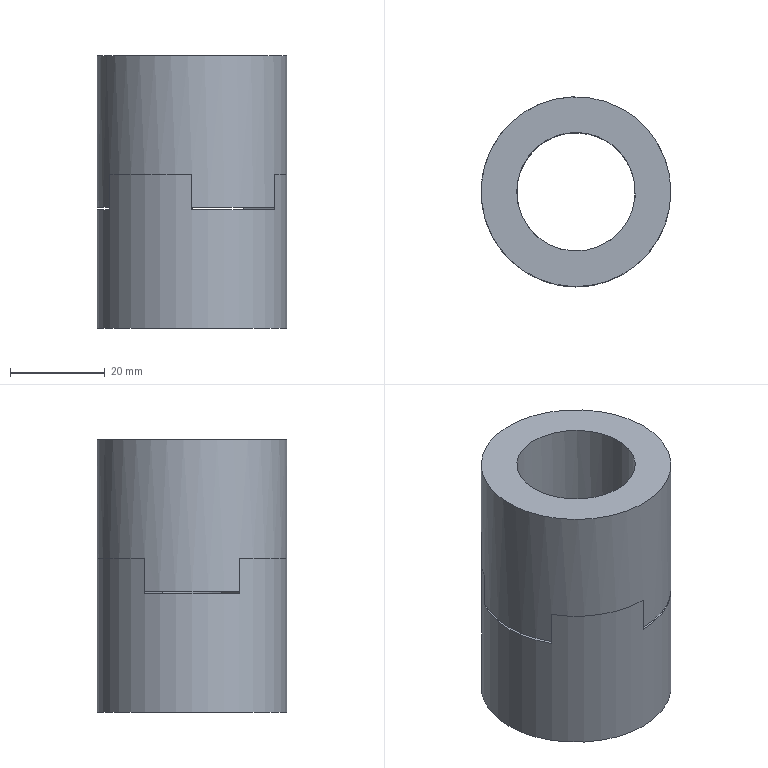Part | NX | 2 solids | 30 faces | box 40 x 40 x 57.5 mm | volume 43840 mm3 | plane 26 | cylinder 4 | commonest cylinder face diameters 25 x2 40 x2
STEP:
#1=CARTESIAN_POINT('',(740.769,-282.606,215.5));
#2=VERTEX_POINT('',#1);
#3=CARTESIAN_POINT('',(751.594,-276.356,215.5));
#4=VERTEX_POINT('',#3);
#5=CARTESIAN_POINT('',(751.594,-288.856,215.5));
#6=DIRECTION('',(0.,0.,-1.));
#7=DIRECTION('',(-1.,0.,0.));
#8=AXIS2_PLACEMENT_3D('',#5,#6,#7);
#9=CIRCLE('',#8,12.5);
#10=EDGE_CURVE('',#2,#4,#9,.T.);
#11=ORIENTED_EDGE('',*,*,#10,.F.);
#12=CARTESIAN_POINT('',(734.274,-278.856,215.5));
#13=VERTEX_POINT('',#12);
#14=CARTESIAN_POINT('',(734.274,-278.856,215.5));
#15=DIRECTION('',(0.866,-0.5,0.));
#16=VECTOR('',#15,1.);
#17=LINE('',#14,#16);
#18=EDGE_CURVE('',#13,#2,#17,.T.);
#19=ORIENTED_EDGE('',*,*,#18,.F.);
#20=CARTESIAN_POINT('',(751.594,-268.856,215.5));
#21=VERTEX_POINT('',#20);
#22=CARTESIAN_POINT('',(751.594,-288.856,215.5));
#23=DIRECTION('',(0.,0.,-1.));
#24=DIRECTION('',(-1.,0.,0.));
#25=AXIS2_PLACEMENT_3D('',#22,#23,#24);
#26=CIRCLE('',#25,20.);
#27=EDGE_CURVE('',#13,#21,#26,.T.);
#28=ORIENTED_EDGE('',*,*,#27,.T.);
#29=CARTESIAN_POINT('',(751.594,-276.356,215.5));
#30=DIRECTION('',(0.,1.,0.));
#31=VECTOR('',#30,1.);
#32=LINE('',#29,#31);
#33=EDGE_CURVE('',#4,#21,#32,.T.);
#34=ORIENTED_EDGE('',*,*,#33,.F.);
#35=EDGE_LOOP('',(#11,#19,#28,#34));
#36=FACE_OUTER_BOUND('',#35,.T.);
#37=CARTESIAN_POINT('',(751.594,-288.856,215.5));
#38=DIRECTION('',(0.,0.,-1.));
#39=DIRECTION('',(1.,0.,0.));
#40=AXIS2_PLACEMENT_3D('',#37,#38,#39);
#41=PLANE('',#40);
#42=ADVANCED_FACE('',(#36),#41,.T.);
#43=CARTESIAN_POINT('',(762.42,-282.606,215.5));
#44=VERTEX_POINT('',#43);
#45=CARTESIAN_POINT('',(762.42,-295.106,215.5));
#46=VERTEX_POINT('',#45);
#47=CARTESIAN_POINT('',(751.594,-288.856,215.5));
#48=DIRECTION('',(0.,0.,-1.));
#49=DIRECTION('',(-1.,0.,0.));
#50=AXIS2_PLACEMENT_3D('',#47,#48,#49);
#51=CIRCLE('',#50,12.5);
#52=EDGE_CURVE('',#44,#46,#51,.T.);
#53=ORIENTED_EDGE('',*,*,#52,.F.);
#54=CARTESIAN_POINT('',(768.915,-278.856,215.5));
#55=VERTEX_POINT('',#54);
#56=CARTESIAN_POINT('',(768.915,-278.856,215.5));
#57=DIRECTION('',(-0.866,-0.5,0.));
#58=VECTOR('',#57,1.);
#59=LINE('',#56,#58);
#60=EDGE_CURVE('',#55,#44,#59,.T.);
#61=ORIENTED_EDGE('',*,*,#60,.F.);
#62=CARTESIAN_POINT('',(768.915,-298.856,215.5));
#63=VERTEX_POINT('',#62);
#64=CARTESIAN_POINT('',(751.594,-288.856,215.5));
#65=DIRECTION('',(0.,0.,-1.));
#66=DIRECTION('',(-1.,0.,0.));
#67=AXIS2_PLACEMENT_3D('',#64,#65,#66);
#68=CIRCLE('',#67,20.);
#69=EDGE_CURVE('',#55,#63,#68,.T.);
#70=ORIENTED_EDGE('',*,*,#69,.T.);
#71=CARTESIAN_POINT('',(762.42,-295.106,215.5));
#72=DIRECTION('',(0.866,-0.5,0.));
#73=VECTOR('',#72,1.);
#74=LINE('',#71,#73);
#75=EDGE_CURVE('',#46,#63,#74,.T.);
#76=ORIENTED_EDGE('',*,*,#75,.F.);
#77=EDGE_LOOP('',(#53,#61,#70,#76));
#78=FACE_OUTER_BOUND('',#77,.T.);
#79=CARTESIAN_POINT('',(751.594,-288.856,215.5));
#80=DIRECTION('',(0.,0.,-1.));
#81=DIRECTION('',(1.,0.,0.));
#82=AXIS2_PLACEMENT_3D('',#79,#80,#81);
#83=PLANE('',#82);
#84=ADVANCED_FACE('',(#78),#83,.T.);
#85=CARTESIAN_POINT('',(751.594,-301.356,215.5));
#86=VERTEX_POINT('',#85);
#87=CARTESIAN_POINT('',(740.769,-295.106,215.5));
#88=VERTEX_POINT('',#87);
#89=CARTESIAN_POINT('',(751.594,-288.856,215.5));
#90=DIRECTION('',(0.,0.,-1.));
#91=DIRECTION('',(-1.,0.,0.));
#92=AXIS2_PLACEMENT_3D('',#89,#90,#91);
#93=CIRCLE('',#92,12.5);
#94=EDGE_CURVE('',#86,#88,#93,.T.);
#95=ORIENTED_EDGE('',*,*,#94,.F.);
#96=CARTESIAN_POINT('',(751.594,-308.856,215.5));
#97=VERTEX_POINT('',#96);
#98=CARTESIAN_POINT('',(751.594,-308.856,215.5));
#99=DIRECTION('',(0.,1.,0.));
#100=VECTOR('',#99,1.);
#101=LINE('',#98,#100);
#102=EDGE_CURVE('',#97,#86,#101,.T.);
#103=ORIENTED_EDGE('',*,*,#102,.F.);
#104=CARTESIAN_POINT('',(734.274,-298.856,215.5));
#105=VERTEX_POINT('',#104);
#106=CARTESIAN_POINT('',(751.594,-288.856,215.5));
#107=DIRECTION('',(0.,0.,-1.));
#108=DIRECTION('',(-1.,0.,0.));
#109=AXIS2_PLACEMENT_3D('',#106,#107,#108);
#110=CIRCLE('',#109,20.);
#111=EDGE_CURVE('',#97,#105,#110,.T.);
#112=ORIENTED_EDGE('',*,*,#111,.T.);
#113=CARTESIAN_POINT('',(740.769,-295.106,215.5));
#114=DIRECTION('',(-0.866,-0.5,0.));
#115=VECTOR('',#114,1.);
#116=LINE('',#113,#115);
#117=EDGE_CURVE('',#88,#105,#116,.T.);
#118=ORIENTED_EDGE('',*,*,#117,.F.);
#119=EDGE_LOOP('',(#95,#103,#112,#118));
#120=FACE_OUTER_BOUND('',#119,.T.);
#121=CARTESIAN_POINT('',(751.594,-288.856,215.5));
#122=DIRECTION('',(0.,0.,-1.));
#123=DIRECTION('',(1.,0.,0.));
#124=AXIS2_PLACEMENT_3D('',#121,#122,#123);
#125=PLANE('',#124);
#126=ADVANCED_FACE('',(#120),#125,.T.);
#127=CARTESIAN_POINT('',(771.594,-288.856,240.5));
#128=VERTEX_POINT('',#127);
#129=CARTESIAN_POINT('',(751.594,-288.856,240.5));
#130=DIRECTION('',(0.,0.,1.));
#131=DIRECTION('',(1.,0.,0.));
#132=AXIS2_PLACEMENT_3D('',#129,#130,#131);
#133=CIRCLE('',#132,20.);
#134=EDGE_CURVE('',#128,#128,#133,.T.);
#135=ORIENTED_EDGE('',*,*,#134,.F.);
#136=EDGE_LOOP('',(#135));
#137=FACE_BOUND('',#136,.T.);
#138=ORIENTED_EDGE('',*,*,#111,.F.);
#139=CARTESIAN_POINT('',(751.594,-308.856,208.5));
#140=VERTEX_POINT('',#139);
#141=CARTESIAN_POINT('',(751.594,-308.856,215.5));
#142=DIRECTION('',(0.,0.,-1.));
#143=VECTOR('',#142,1.);
#144=LINE('',#141,#143);
#145=EDGE_CURVE('',#97,#140,#144,.T.);
#146=ORIENTED_EDGE('',*,*,#145,.T.);
#147=CARTESIAN_POINT('',(768.915,-298.856,208.5));
#148=VERTEX_POINT('',#147);
#149=CARTESIAN_POINT('',(751.594,-288.856,208.5));
#150=DIRECTION('',(0.,0.,1.));
#151=DIRECTION('',(1.,0.,0.));
#152=AXIS2_PLACEMENT_3D('',#149,#150,#151);
#153=CIRCLE('',#152,20.);
#154=EDGE_CURVE('',#140,#148,#153,.T.);
#155=ORIENTED_EDGE('',*,*,#154,.T.);
#156=CARTESIAN_POINT('',(768.915,-298.856,215.5));
#157=DIRECTION('',(0.,0.,-1.));
#158=VECTOR('',#157,1.);
#159=LINE('',#156,#158);
#160=EDGE_CURVE('',#63,#148,#159,.T.);
#161=ORIENTED_EDGE('',*,*,#160,.F.);
#162=ORIENTED_EDGE('',*,*,#69,.F.);
#163=CARTESIAN_POINT('',(768.915,-278.856,208.5));
#164=VERTEX_POINT('',#163);
#165=CARTESIAN_POINT('',(768.915,-278.856,215.5));
#166=DIRECTION('',(0.,0.,-1.));
#167=VECTOR('',#166,1.);
#168=LINE('',#165,#167);
#169=EDGE_CURVE('',#55,#164,#168,.T.);
#170=ORIENTED_EDGE('',*,*,#169,.T.);
#171=CARTESIAN_POINT('',(751.594,-268.856,208.5));
#172=VERTEX_POINT('',#171);
#173=CARTESIAN_POINT('',(751.594,-288.856,208.5));
#174=DIRECTION('',(0.,0.,1.));
#175=DIRECTION('',(1.,0.,0.));
#176=AXIS2_PLACEMENT_3D('',#173,#174,#175);
#177=CIRCLE('',#176,20.);
#178=EDGE_CURVE('',#164,#172,#177,.T.);
#179=ORIENTED_EDGE('',*,*,#178,.T.);
#180=CARTESIAN_POINT('',(751.594,-268.856,215.5));
#181=DIRECTION('',(0.,0.,-1.));
#182=VECTOR('',#181,1.);
#183=LINE('',#180,#182);
#184=EDGE_CURVE('',#21,#172,#183,.T.);
#185=ORIENTED_EDGE('',*,*,#184,.F.);
#186=ORIENTED_EDGE('',*,*,#27,.F.);
#187=CARTESIAN_POINT('',(734.274,-278.856,208.5));
#188=VERTEX_POINT('',#187);
#189=CARTESIAN_POINT('',(734.274,-278.856,215.5));
#190=DIRECTION('',(0.,0.,-1.));
#191=VECTOR('',#190,1.);
#192=LINE('',#189,#191);
#193=EDGE_CURVE('',#13,#188,#192,.T.);
#194=ORIENTED_EDGE('',*,*,#193,.T.);
#195=CARTESIAN_POINT('',(734.274,-298.856,208.5));
#196=VERTEX_POINT('',#195);
#197=CARTESIAN_POINT('',(751.594,-288.856,208.5));
#198=DIRECTION('',(0.,0.,1.));
#199=DIRECTION('',(1.,0.,0.));
#200=AXIS2_PLACEMENT_3D('',#197,#198,#199);
#201=CIRCLE('',#200,20.);
#202=EDGE_CURVE('',#188,#196,#201,.T.);
#203=ORIENTED_EDGE('',*,*,#202,.T.);
#204=CARTESIAN_POINT('',(734.274,-298.856,215.5));
#205=DIRECTION('',(0.,0.,-1.));
#206=VECTOR('',#205,1.);
#207=LINE('',#204,#206);
#208=EDGE_CURVE('',#105,#196,#207,.T.);
#209=ORIENTED_EDGE('',*,*,#208,.F.);
#210=EDGE_LOOP('',(#138,#146,#155,#161,#162,#170,#179,#185,#186,#194,#203,#209));
#211=FACE_BOUND('',#210,.T.);
#212=CARTESIAN_POINT('',(751.594,-288.856,240.5));
#213=DIRECTION('',(0.,0.,-1.));
#214=DIRECTION('',(1.,0.,0.));
#215=AXIS2_PLACEMENT_3D('',#212,#213,#214);
#216=CYLINDRICAL_SURFACE('',#215,20.);
#217=ADVANCED_FACE('',(#137,#211),#216,.T.);
#218=CARTESIAN_POINT('',(739.094,-288.856,240.5));
#219=VERTEX_POINT('',#218);
#220=CARTESIAN_POINT('',(751.594,-288.856,240.5));
#221=DIRECTION('',(0.,0.,-1.));
#222=DIRECTION('',(-1.,0.,0.));
#223=AXIS2_PLACEMENT_3D('',#220,#221,#222);
#224=CIRCLE('',#223,12.5);
#225=EDGE_CURVE('',#219,#219,#224,.T.);
#226=ORIENTED_EDGE('',*,*,#225,.T.);
#227=EDGE_LOOP('',(#226));
#228=FACE_BOUND('',#227,.T.);
#229=ORIENTED_EDGE('',*,*,#134,.T.);
#230=EDGE_LOOP('',(#229));
#231=FACE_BOUND('',#230,.T.);
#232=CARTESIAN_POINT('',(751.594,-288.856,240.5));
#233=DIRECTION('',(0.,0.,1.));
#234=DIRECTION('',(-1.,0.,0.));
#235=AXIS2_PLACEMENT_3D('',#232,#233,#234);
#236=PLANE('',#235);
#237=ADVANCED_FACE('',(#228,#231),#236,.T.);
#238=CARTESIAN_POINT('',(751.594,-301.356,208.5));
#239=VERTEX_POINT('',#238);
#240=CARTESIAN_POINT('',(751.594,-308.856,208.5));
#241=DIRECTION('',(0.,1.,0.));
#242=VECTOR('',#241,1.);
#243=LINE('',#240,#242);
#244=EDGE_CURVE('',#140,#239,#243,.T.);
#245=ORIENTED_EDGE('',*,*,#244,.F.);
#246=ORIENTED_EDGE('',*,*,#145,.F.);
#247=ORIENTED_EDGE('',*,*,#102,.T.);
#248=CARTESIAN_POINT('',(751.594,-301.356,215.5));
#249=DIRECTION('',(0.,0.,-1.));
#250=VECTOR('',#249,1.);
#251=LINE('',#248,#250);
#252=EDGE_CURVE('',#86,#239,#251,.T.);
#253=ORIENTED_EDGE('',*,*,#252,.T.);
#254=EDGE_LOOP('',(#245,#246,#247,#253));
#255=FACE_OUTER_BOUND('',#254,.T.);
#256=CARTESIAN_POINT('',(751.594,-308.856,215.5));
#257=DIRECTION('',(-1.,0.,0.));
#258=DIRECTION('',(0.,0.,-1.));
#259=AXIS2_PLACEMENT_3D('',#256,#257,#258);
#260=PLANE('',#259);
#261=ADVANCED_FACE('',(#255),#260,.T.);
#262=CARTESIAN_POINT('',(762.42,-295.106,208.5));
#263=VERTEX_POINT('',#262);
#264=CARTESIAN_POINT('',(762.42,-295.106,208.5));
#265=DIRECTION('',(0.866,-0.5,0.));
#266=VECTOR('',#265,1.);
#267=LINE('',#264,#266);
#268=EDGE_CURVE('',#263,#148,#267,.T.);
#269=ORIENTED_EDGE('',*,*,#268,.F.);
#270=CARTESIAN_POINT('',(762.42,-295.106,215.5));
#271=DIRECTION('',(0.,0.,-1.));
#272=VECTOR('',#271,1.);
#273=LINE('',#270,#272);
#274=EDGE_CURVE('',#46,#263,#273,.T.);
#275=ORIENTED_EDGE('',*,*,#274,.F.);
#276=ORIENTED_EDGE('',*,*,#75,.T.);
#277=ORIENTED_EDGE('',*,*,#160,.T.);
#278=EDGE_LOOP('',(#269,#275,#276,#277));
#279=FACE_OUTER_BOUND('',#278,.T.);
#280=CARTESIAN_POINT('',(762.42,-295.106,215.5));
#281=DIRECTION('',(0.5,0.866,0.));
#282=DIRECTION('',(0.866,-0.5,0.));
#283=AXIS2_PLACEMENT_3D('',#280,#281,#282);
#284=PLANE('',#283);
#285=ADVANCED_FACE('',(#279),#284,.T.);
#286=CARTESIAN_POINT('',(751.594,-288.856,208.5));
#287=DIRECTION('',(0.,0.,1.));
#288=DIRECTION('',(1.,0.,0.));
#289=AXIS2_PLACEMENT_3D('',#286,#287,#288);
#290=CIRCLE('',#289,12.5);
#291=EDGE_CURVE('',#239,#263,#290,.T.);
#292=ORIENTED_EDGE('',*,*,#291,.F.);
#293=ORIENTED_EDGE('',*,*,#252,.F.);
#294=ORIENTED_EDGE('',*,*,#94,.T.);
#295=CARTESIAN_POINT('',(740.769,-295.106,208.5));
#296=VERTEX_POINT('',#295);
#297=CARTESIAN_POINT('',(740.769,-295.106,215.5));
#298=DIRECTION('',(0.,0.,-1.));
#299=VECTOR('',#298,1.);
#300=LINE('',#297,#299);
#301=EDGE_CURVE('',#88,#296,#300,.T.);
#302=ORIENTED_EDGE('',*,*,#301,.T.);
#303=CARTESIAN_POINT('',(740.769,-282.606,208.5));
#304=VERTEX_POINT('',#303);
#305=CARTESIAN_POINT('',(751.594,-288.856,208.5));
#306=DIRECTION('',(0.,0.,1.));
#307=DIRECTION('',(1.,0.,0.));
#308=AXIS2_PLACEMENT_3D('',#305,#306,#307);
#309=CIRCLE('',#308,12.5);
#310=EDGE_CURVE('',#304,#296,#309,.T.);
#311=ORIENTED_EDGE('',*,*,#310,.F.);
#312=CARTESIAN_POINT('',(740.769,-282.606,215.5));
#313=DIRECTION('',(0.,0.,-1.));
#314=VECTOR('',#313,1.);
#315=LINE('',#312,#314);
#316=EDGE_CURVE('',#2,#304,#315,.T.);
#317=ORIENTED_EDGE('',*,*,#316,.F.);
#318=ORIENTED_EDGE('',*,*,#10,.T.);
#319=CARTESIAN_POINT('',(751.594,-276.356,208.5));
#320=VERTEX_POINT('',#319);
#321=CARTESIAN_POINT('',(751.594,-276.356,215.5));
#322=DIRECTION('',(0.,0.,-1.));
#323=VECTOR('',#322,1.);
#324=LINE('',#321,#323);
#325=EDGE_CURVE('',#4,#320,#324,.T.);
#326=ORIENTED_EDGE('',*,*,#325,.T.);
#327=CARTESIAN_POINT('',(762.42,-282.606,208.5));
#328=VERTEX_POINT('',#327);
#329=CARTESIAN_POINT('',(751.594,-288.856,208.5));
#330=DIRECTION('',(0.,0.,1.));
#331=DIRECTION('',(1.,0.,0.));
#332=AXIS2_PLACEMENT_3D('',#329,#330,#331);
#333=CIRCLE('',#332,12.5);
#334=EDGE_CURVE('',#328,#320,#333,.T.);
#335=ORIENTED_EDGE('',*,*,#334,.F.);
#336=CARTESIAN_POINT('',(762.42,-282.606,215.5));
#337=DIRECTION('',(0.,0.,-1.));
#338=VECTOR('',#337,1.);
#339=LINE('',#336,#338);
#340=EDGE_CURVE('',#44,#328,#339,.T.);
#341=ORIENTED_EDGE('',*,*,#340,.F.);
#342=ORIENTED_EDGE('',*,*,#52,.T.);
#343=ORIENTED_EDGE('',*,*,#274,.T.);
#344=EDGE_LOOP('',(#292,#293,#294,#302,#311,#317,#318,#326,#335,#341,#342,#343));
#345=FACE_BOUND('',#344,.T.);
#346=ORIENTED_EDGE('',*,*,#225,.F.);
#347=EDGE_LOOP('',(#346));
#348=FACE_BOUND('',#347,.T.);
#349=CARTESIAN_POINT('',(751.594,-288.856,215.5));
#350=DIRECTION('',(0.,0.,-1.));
#351=DIRECTION('',(1.,0.,0.));
#352=AXIS2_PLACEMENT_3D('',#349,#350,#351);
#353=CYLINDRICAL_SURFACE('',#352,12.5);
#354=ADVANCED_FACE('',(#345,#348),#353,.F.);
#355=ORIENTED_EDGE('',*,*,#244,.T.);
#356=ORIENTED_EDGE('',*,*,#291,.T.);
#357=ORIENTED_EDGE('',*,*,#268,.T.);
#358=ORIENTED_EDGE('',*,*,#154,.F.);
#359=EDGE_LOOP('',(#355,#356,#357,#358));
#360=FACE_OUTER_BOUND('',#359,.T.);
#361=CARTESIAN_POINT('',(751.594,-288.856,208.5));
#362=DIRECTION('',(0.,0.,1.));
#363=DIRECTION('',(-1.,0.,0.));
#364=AXIS2_PLACEMENT_3D('',#361,#362,#363);
#365=PLANE('',#364);
#366=ADVANCED_FACE('',(#360),#365,.F.);
#367=CARTESIAN_POINT('',(740.769,-295.106,208.5));
#368=DIRECTION('',(-0.866,-0.5,0.));
#369=VECTOR('',#368,1.);
#370=LINE('',#367,#369);
#371=EDGE_CURVE('',#296,#196,#370,.T.);
#372=ORIENTED_EDGE('',*,*,#371,.F.);
#373=ORIENTED_EDGE('',*,*,#301,.F.);
#374=ORIENTED_EDGE('',*,*,#117,.T.);
#375=ORIENTED_EDGE('',*,*,#208,.T.);
#376=EDGE_LOOP('',(#372,#373,#374,#375));
#377=FACE_OUTER_BOUND('',#376,.T.);
#378=CARTESIAN_POINT('',(740.769,-295.106,215.5));
#379=DIRECTION('',(0.5,-0.866,0.));
#380=DIRECTION('',(-0.866,-0.5,0.));
#381=AXIS2_PLACEMENT_3D('',#378,#379,#380);
#382=PLANE('',#381);
#383=ADVANCED_FACE('',(#377),#382,.T.);
#384=CARTESIAN_POINT('',(734.274,-278.856,208.5));
#385=DIRECTION('',(0.866,-0.5,0.));
#386=VECTOR('',#385,1.);
#387=LINE('',#384,#386);
#388=EDGE_CURVE('',#188,#304,#387,.T.);
#389=ORIENTED_EDGE('',*,*,#388,.F.);
#390=ORIENTED_EDGE('',*,*,#193,.F.);
#391=ORIENTED_EDGE('',*,*,#18,.T.);
#392=ORIENTED_EDGE('',*,*,#316,.T.);
#393=EDGE_LOOP('',(#389,#390,#391,#392));
#394=FACE_OUTER_BOUND('',#393,.T.);
#395=CARTESIAN_POINT('',(734.274,-278.856,215.5));
#396=DIRECTION('',(0.5,0.866,0.));
#397=DIRECTION('',(0.866,-0.5,0.));
#398=AXIS2_PLACEMENT_3D('',#395,#396,#397);
#399=PLANE('',#398);
#400=ADVANCED_FACE('',(#394),#399,.T.);
#401=ORIENTED_EDGE('',*,*,#371,.T.);
#402=ORIENTED_EDGE('',*,*,#202,.F.);
#403=ORIENTED_EDGE('',*,*,#388,.T.);
#404=ORIENTED_EDGE('',*,*,#310,.T.);
#405=EDGE_LOOP('',(#401,#402,#403,#404));
#406=FACE_OUTER_BOUND('',#405,.T.);
#407=CARTESIAN_POINT('',(751.594,-288.856,208.5));
#408=DIRECTION('',(0.,0.,1.));
#409=DIRECTION('',(-1.,0.,0.));
#410=AXIS2_PLACEMENT_3D('',#407,#408,#409);
#411=PLANE('',#410);
#412=ADVANCED_FACE('',(#406),#411,.F.);
#413=CARTESIAN_POINT('',(751.594,-276.356,208.5));
#414=DIRECTION('',(0.,1.,0.));
#415=VECTOR('',#414,1.);
#416=LINE('',#413,#415);
#417=EDGE_CURVE('',#320,#172,#416,.T.);
#418=ORIENTED_EDGE('',*,*,#417,.F.);
#419=ORIENTED_EDGE('',*,*,#325,.F.);
#420=ORIENTED_EDGE('',*,*,#33,.T.);
#421=ORIENTED_EDGE('',*,*,#184,.T.);
#422=EDGE_LOOP('',(#418,#419,#420,#421));
#423=FACE_OUTER_BOUND('',#422,.T.);
#424=CARTESIAN_POINT('',(751.594,-276.356,215.5));
#425=DIRECTION('',(-1.,0.,0.));
#426=DIRECTION('',(0.,0.,-1.));
#427=AXIS2_PLACEMENT_3D('',#424,#425,#426);
#428=PLANE('',#427);
#429=ADVANCED_FACE('',(#423),#428,.T.);
#430=CARTESIAN_POINT('',(768.915,-278.856,208.5));
#431=DIRECTION('',(-0.866,-0.5,0.));
#432=VECTOR('',#431,1.);
#433=LINE('',#430,#432);
#434=EDGE_CURVE('',#164,#328,#433,.T.);
#435=ORIENTED_EDGE('',*,*,#434,.F.);
#436=ORIENTED_EDGE('',*,*,#169,.F.);
#437=ORIENTED_EDGE('',*,*,#60,.T.);
#438=ORIENTED_EDGE('',*,*,#340,.T.);
#439=EDGE_LOOP('',(#435,#436,#437,#438));
#440=FACE_OUTER_BOUND('',#439,.T.);
#441=CARTESIAN_POINT('',(768.915,-278.856,215.5));
#442=DIRECTION('',(0.5,-0.866,0.));
#443=DIRECTION('',(-0.866,-0.5,0.));
#444=AXIS2_PLACEMENT_3D('',#441,#442,#443);
#445=PLANE('',#444);
#446=ADVANCED_FACE('',(#440),#445,.T.);
#447=ORIENTED_EDGE('',*,*,#417,.T.);
#448=ORIENTED_EDGE('',*,*,#178,.F.);
#449=ORIENTED_EDGE('',*,*,#434,.T.);
#450=ORIENTED_EDGE('',*,*,#334,.T.);
#451=EDGE_LOOP('',(#447,#448,#449,#450));
#452=FACE_OUTER_BOUND('',#451,.T.);
#453=CARTESIAN_POINT('',(751.594,-288.856,208.5));
#454=DIRECTION('',(0.,0.,1.));
#455=DIRECTION('',(-1.,0.,0.));
#456=AXIS2_PLACEMENT_3D('',#453,#454,#455);
#457=PLANE('',#456);
#458=ADVANCED_FACE('',(#452),#457,.F.);
#459=CLOSED_SHELL('',(#42,#84,#126,#217,#237,#261,#285,#354,#366,#383,#400,#412,#429,#446,#458));
#460=MANIFOLD_SOLID_BREP('',#459);
#461=CARTESIAN_POINT('',(740.769,-295.106,208.));
#462=VERTEX_POINT('',#461);
#463=CARTESIAN_POINT('',(734.274,-298.856,208.));
#464=VERTEX_POINT('',#463);
#465=CARTESIAN_POINT('',(740.769,-295.106,208.));
#466=DIRECTION('',(-0.866,-0.5,0.));
#467=VECTOR('',#466,1.);
#468=LINE('',#465,#467);
#469=EDGE_CURVE('',#462,#464,#468,.T.);
#470=ORIENTED_EDGE('',*,*,#469,.F.);
#471=CARTESIAN_POINT('',(740.769,-282.606,208.));
#472=VERTEX_POINT('',#471);
#473=CARTESIAN_POINT('',(751.594,-288.856,208.));
#474=DIRECTION('',(0.,0.,1.));
#475=DIRECTION('',(1.,0.,0.));
#476=AXIS2_PLACEMENT_3D('',#473,#474,#475);
#477=CIRCLE('',#476,12.5);
#478=EDGE_CURVE('',#472,#462,#477,.T.);
#479=ORIENTED_EDGE('',*,*,#478,.F.);
#480=CARTESIAN_POINT('',(734.274,-278.856,208.));
#481=VERTEX_POINT('',#480);
#482=CARTESIAN_POINT('',(734.274,-278.856,208.));
#483=DIRECTION('',(0.866,-0.5,0.));
#484=VECTOR('',#483,1.);
#485=LINE('',#482,#484);
#486=EDGE_CURVE('',#481,#472,#485,.T.);
#487=ORIENTED_EDGE('',*,*,#486,.F.);
#488=CARTESIAN_POINT('',(751.594,-288.856,208.));
#489=DIRECTION('',(0.,0.,1.));
#490=DIRECTION('',(1.,0.,0.));
#491=AXIS2_PLACEMENT_3D('',#488,#489,#490);
#492=CIRCLE('',#491,20.);
#493=EDGE_CURVE('',#481,#464,#492,.T.);
#494=ORIENTED_EDGE('',*,*,#493,.T.);
#495=EDGE_LOOP('',(#470,#479,#487,#494));
#496=FACE_OUTER_BOUND('',#495,.T.);
#497=CARTESIAN_POINT('',(751.594,-288.856,208.));
#498=DIRECTION('',(0.,0.,1.));
#499=DIRECTION('',(-1.,0.,0.));
#500=AXIS2_PLACEMENT_3D('',#497,#498,#499);
#501=PLANE('',#500);
#502=ADVANCED_FACE('',(#496),#501,.T.);
#503=CARTESIAN_POINT('',(751.594,-308.856,208.));
#504=VERTEX_POINT('',#503);
#505=CARTESIAN_POINT('',(751.594,-301.356,208.));
#506=VERTEX_POINT('',#505);
#507=CARTESIAN_POINT('',(751.594,-308.856,208.));
#508=DIRECTION('',(0.,1.,0.));
#509=VECTOR('',#508,1.);
#510=LINE('',#507,#509);
#511=EDGE_CURVE('',#504,#506,#510,.T.);
#512=ORIENTED_EDGE('',*,*,#511,.F.);
#513=CARTESIAN_POINT('',(768.915,-298.856,208.));
#514=VERTEX_POINT('',#513);
#515=CARTESIAN_POINT('',(751.594,-288.856,208.));
#516=DIRECTION('',(0.,0.,1.));
#517=DIRECTION('',(1.,0.,0.));
#518=AXIS2_PLACEMENT_3D('',#515,#516,#517);
#519=CIRCLE('',#518,20.);
#520=EDGE_CURVE('',#504,#514,#519,.T.);
#521=ORIENTED_EDGE('',*,*,#520,.T.);
#522=CARTESIAN_POINT('',(762.42,-295.106,208.));
#523=VERTEX_POINT('',#522);
#524=CARTESIAN_POINT('',(762.42,-295.106,208.));
#525=DIRECTION('',(0.866,-0.5,0.));
#526=VECTOR('',#525,1.);
#527=LINE('',#524,#526);
#528=EDGE_CURVE('',#523,#514,#527,.T.);
#529=ORIENTED_EDGE('',*,*,#528,.F.);
#530=CARTESIAN_POINT('',(751.594,-288.856,208.));
#531=DIRECTION('',(0.,0.,1.));
#532=DIRECTION('',(1.,0.,0.));
#533=AXIS2_PLACEMENT_3D('',#530,#531,#532);
#534=CIRCLE('',#533,12.5);
#535=EDGE_CURVE('',#506,#523,#534,.T.);
#536=ORIENTED_EDGE('',*,*,#535,.F.);
#537=EDGE_LOOP('',(#512,#521,#529,#536));
#538=FACE_OUTER_BOUND('',#537,.T.);
#539=CARTESIAN_POINT('',(751.594,-288.856,208.));
#540=DIRECTION('',(0.,0.,1.));
#541=DIRECTION('',(-1.,0.,0.));
#542=AXIS2_PLACEMENT_3D('',#539,#540,#541);
#543=PLANE('',#542);
#544=ADVANCED_FACE('',(#538),#543,.T.);
#545=CARTESIAN_POINT('',(751.594,-276.356,208.));
#546=VERTEX_POINT('',#545);
#547=CARTESIAN_POINT('',(751.594,-268.856,208.));
#548=VERTEX_POINT('',#547);
#549=CARTESIAN_POINT('',(751.594,-276.356,208.));
#550=DIRECTION('',(0.,1.,0.));
#551=VECTOR('',#550,1.);
#552=LINE('',#549,#551);
#553=EDGE_CURVE('',#546,#548,#552,.T.);
#554=ORIENTED_EDGE('',*,*,#553,.F.);
#555=CARTESIAN_POINT('',(762.42,-282.606,208.));
#556=VERTEX_POINT('',#555);
#557=CARTESIAN_POINT('',(751.594,-288.856,208.));
#558=DIRECTION('',(0.,0.,1.));
#559=DIRECTION('',(1.,0.,0.));
#560=AXIS2_PLACEMENT_3D('',#557,#558,#559);
#561=CIRCLE('',#560,12.5);
#562=EDGE_CURVE('',#556,#546,#561,.T.);
#563=ORIENTED_EDGE('',*,*,#562,.F.);
#564=CARTESIAN_POINT('',(768.915,-278.856,208.));
#565=VERTEX_POINT('',#564);
#566=CARTESIAN_POINT('',(768.915,-278.856,208.));
#567=DIRECTION('',(-0.866,-0.5,0.));
#568=VECTOR('',#567,1.);
#569=LINE('',#566,#568);
#570=EDGE_CURVE('',#565,#556,#569,.T.);
#571=ORIENTED_EDGE('',*,*,#570,.F.);
#572=CARTESIAN_POINT('',(751.594,-288.856,208.));
#573=DIRECTION('',(0.,0.,1.));
#574=DIRECTION('',(1.,0.,0.));
#575=AXIS2_PLACEMENT_3D('',#572,#573,#574);
#576=CIRCLE('',#575,20.);
#577=EDGE_CURVE('',#565,#548,#576,.T.);
#578=ORIENTED_EDGE('',*,*,#577,.T.);
#579=EDGE_LOOP('',(#554,#563,#571,#578));
#580=FACE_OUTER_BOUND('',#579,.T.);
#581=CARTESIAN_POINT('',(751.594,-288.856,208.));
#582=DIRECTION('',(0.,0.,1.));
#583=DIRECTION('',(-1.,0.,0.));
#584=AXIS2_PLACEMENT_3D('',#581,#582,#583);
#585=PLANE('',#584);
#586=ADVANCED_FACE('',(#580),#585,.T.);
#587=CARTESIAN_POINT('',(771.594,-288.856,183.));
#588=VERTEX_POINT('',#587);
#589=CARTESIAN_POINT('',(751.594,-288.856,183.));
#590=DIRECTION('',(0.,0.,1.));
#591=DIRECTION('',(1.,0.,0.));
#592=AXIS2_PLACEMENT_3D('',#589,#590,#591);
#593=CIRCLE('',#592,20.);
#594=EDGE_CURVE('',#588,#588,#593,.T.);
#595=ORIENTED_EDGE('',*,*,#594,.T.);
#596=EDGE_LOOP('',(#595));
#597=FACE_BOUND('',#596,.T.);
#598=ORIENTED_EDGE('',*,*,#577,.F.);
#599=CARTESIAN_POINT('',(768.915,-278.856,215.5));
#600=VERTEX_POINT('',#599);
#601=CARTESIAN_POINT('',(768.915,-278.856,215.5));
#602=DIRECTION('',(0.,0.,-1.));
#603=VECTOR('',#602,1.);
#604=LINE('',#601,#603);
#605=EDGE_CURVE('',#600,#565,#604,.T.);
#606=ORIENTED_EDGE('',*,*,#605,.F.);
#607=CARTESIAN_POINT('',(768.915,-298.856,215.5));
#608=VERTEX_POINT('',#607);
#609=CARTESIAN_POINT('',(751.594,-288.856,215.5));
#610=DIRECTION('',(0.,0.,1.));
#611=DIRECTION('',(1.,0.,0.));
#612=AXIS2_PLACEMENT_3D('',#609,#610,#611);
#613=CIRCLE('',#612,20.);
#614=EDGE_CURVE('',#608,#600,#613,.T.);
#615=ORIENTED_EDGE('',*,*,#614,.F.);
#616=CARTESIAN_POINT('',(768.915,-298.856,215.5));
#617=DIRECTION('',(0.,0.,-1.));
#618=VECTOR('',#617,1.);
#619=LINE('',#616,#618);
#620=EDGE_CURVE('',#608,#514,#619,.T.);
#621=ORIENTED_EDGE('',*,*,#620,.T.);
#622=ORIENTED_EDGE('',*,*,#520,.F.);
#623=CARTESIAN_POINT('',(751.594,-308.856,215.5));
#624=VERTEX_POINT('',#623);
#625=CARTESIAN_POINT('',(751.594,-308.856,215.5));
#626=DIRECTION('',(0.,0.,-1.));
#627=VECTOR('',#626,1.);
#628=LINE('',#625,#627);
#629=EDGE_CURVE('',#624,#504,#628,.T.);
#630=ORIENTED_EDGE('',*,*,#629,.F.);
#631=CARTESIAN_POINT('',(734.274,-298.856,215.5));
#632=VERTEX_POINT('',#631);
#633=CARTESIAN_POINT('',(751.594,-288.856,215.5));
#634=DIRECTION('',(0.,0.,1.));
#635=DIRECTION('',(1.,0.,0.));
#636=AXIS2_PLACEMENT_3D('',#633,#634,#635);
#637=CIRCLE('',#636,20.);
#638=EDGE_CURVE('',#632,#624,#637,.T.);
#639=ORIENTED_EDGE('',*,*,#638,.F.);
#640=CARTESIAN_POINT('',(734.274,-298.856,215.5));
#641=DIRECTION('',(0.,0.,-1.));
#642=VECTOR('',#641,1.);
#643=LINE('',#640,#642);
#644=EDGE_CURVE('',#632,#464,#643,.T.);
#645=ORIENTED_EDGE('',*,*,#644,.T.);
#646=ORIENTED_EDGE('',*,*,#493,.F.);
#647=CARTESIAN_POINT('',(734.274,-278.856,215.5));
#648=VERTEX_POINT('',#647);
#649=CARTESIAN_POINT('',(734.274,-278.856,215.5));
#650=DIRECTION('',(0.,0.,-1.));
#651=VECTOR('',#650,1.);
#652=LINE('',#649,#651);
#653=EDGE_CURVE('',#648,#481,#652,.T.);
#654=ORIENTED_EDGE('',*,*,#653,.F.);
#655=CARTESIAN_POINT('',(751.594,-268.856,215.5));
#656=VERTEX_POINT('',#655);
#657=CARTESIAN_POINT('',(751.594,-288.856,215.5));
#658=DIRECTION('',(0.,0.,1.));
#659=DIRECTION('',(1.,0.,0.));
#660=AXIS2_PLACEMENT_3D('',#657,#658,#659);
#661=CIRCLE('',#660,20.);
#662=EDGE_CURVE('',#656,#648,#661,.T.);
#663=ORIENTED_EDGE('',*,*,#662,.F.);
#664=CARTESIAN_POINT('',(751.594,-268.856,215.5));
#665=DIRECTION('',(0.,0.,-1.));
#666=VECTOR('',#665,1.);
#667=LINE('',#664,#666);
#668=EDGE_CURVE('',#656,#548,#667,.T.);
#669=ORIENTED_EDGE('',*,*,#668,.T.);
#670=EDGE_LOOP('',(#598,#606,#615,#621,#622,#630,#639,#645,#646,#654,#663,#669));
#671=FACE_BOUND('',#670,.T.);
#672=CARTESIAN_POINT('',(751.594,-288.856,183.));
#673=DIRECTION('',(0.,0.,1.));
#674=DIRECTION('',(-1.,0.,0.));
#675=AXIS2_PLACEMENT_3D('',#672,#673,#674);
#676=CYLINDRICAL_SURFACE('',#675,20.);
#677=ADVANCED_FACE('',(#597,#671),#676,.T.);
#678=CARTESIAN_POINT('',(764.094,-288.856,183.));
#679=VERTEX_POINT('',#678);
#680=CARTESIAN_POINT('',(751.594,-288.856,183.));
#681=DIRECTION('',(0.,0.,1.));
#682=DIRECTION('',(1.,0.,0.));
#683=AXIS2_PLACEMENT_3D('',#680,#681,#682);
#684=CIRCLE('',#683,12.5);
#685=EDGE_CURVE('',#679,#679,#684,.T.);
#686=ORIENTED_EDGE('',*,*,#685,.F.);
#687=EDGE_LOOP('',(#686));
#688=FACE_BOUND('',#687,.T.);
#689=ORIENTED_EDGE('',*,*,#562,.T.);
#690=CARTESIAN_POINT('',(751.594,-276.356,215.5));
#691=VERTEX_POINT('',#690);
#692=CARTESIAN_POINT('',(751.594,-276.356,215.5));
#693=DIRECTION('',(0.,0.,-1.));
#694=VECTOR('',#693,1.);
#695=LINE('',#692,#694);
#696=EDGE_CURVE('',#691,#546,#695,.T.);
#697=ORIENTED_EDGE('',*,*,#696,.F.);
#698=CARTESIAN_POINT('',(740.769,-282.606,215.5));
#699=VERTEX_POINT('',#698);
#700=CARTESIAN_POINT('',(751.594,-288.856,215.5));
#701=DIRECTION('',(0.,0.,-1.));
#702=DIRECTION('',(1.,0.,0.));
#703=AXIS2_PLACEMENT_3D('',#700,#701,#702);
#704=CIRCLE('',#703,12.5);
#705=EDGE_CURVE('',#699,#691,#704,.T.);
#706=ORIENTED_EDGE('',*,*,#705,.F.);
#707=CARTESIAN_POINT('',(740.769,-282.606,215.5));
#708=DIRECTION('',(0.,0.,-1.));
#709=VECTOR('',#708,1.);
#710=LINE('',#707,#709);
#711=EDGE_CURVE('',#699,#472,#710,.T.);
#712=ORIENTED_EDGE('',*,*,#711,.T.);
#713=ORIENTED_EDGE('',*,*,#478,.T.);
#714=CARTESIAN_POINT('',(740.769,-295.106,215.5));
#715=VERTEX_POINT('',#714);
#716=CARTESIAN_POINT('',(740.769,-295.106,215.5));
#717=DIRECTION('',(0.,0.,-1.));
#718=VECTOR('',#717,1.);
#719=LINE('',#716,#718);
#720=EDGE_CURVE('',#715,#462,#719,.T.);
#721=ORIENTED_EDGE('',*,*,#720,.F.);
#722=CARTESIAN_POINT('',(751.594,-301.356,215.5));
#723=VERTEX_POINT('',#722);
#724=CARTESIAN_POINT('',(751.594,-288.856,215.5));
#725=DIRECTION('',(0.,0.,-1.));
#726=DIRECTION('',(1.,0.,0.));
#727=AXIS2_PLACEMENT_3D('',#724,#725,#726);
#728=CIRCLE('',#727,12.5);
#729=EDGE_CURVE('',#723,#715,#728,.T.);
#730=ORIENTED_EDGE('',*,*,#729,.F.);
#731=CARTESIAN_POINT('',(751.594,-301.356,215.5));
#732=DIRECTION('',(0.,0.,-1.));
#733=VECTOR('',#732,1.);
#734=LINE('',#731,#733);
#735=EDGE_CURVE('',#723,#506,#734,.T.);
#736=ORIENTED_EDGE('',*,*,#735,.T.);
#737=ORIENTED_EDGE('',*,*,#535,.T.);
#738=CARTESIAN_POINT('',(762.42,-295.106,215.5));
#739=VERTEX_POINT('',#738);
#740=CARTESIAN_POINT('',(762.42,-295.106,215.5));
#741=DIRECTION('',(0.,0.,-1.));
#742=VECTOR('',#741,1.);
#743=LINE('',#740,#742);
#744=EDGE_CURVE('',#739,#523,#743,.T.);
#745=ORIENTED_EDGE('',*,*,#744,.F.);
#746=CARTESIAN_POINT('',(762.42,-282.606,215.5));
#747=VERTEX_POINT('',#746);
#748=CARTESIAN_POINT('',(751.594,-288.856,215.5));
#749=DIRECTION('',(0.,0.,-1.));
#750=DIRECTION('',(1.,0.,0.));
#751=AXIS2_PLACEMENT_3D('',#748,#749,#750);
#752=CIRCLE('',#751,12.5);
#753=EDGE_CURVE('',#747,#739,#752,.T.);
#754=ORIENTED_EDGE('',*,*,#753,.F.);
#755=CARTESIAN_POINT('',(762.42,-282.606,215.5));
#756=DIRECTION('',(0.,0.,-1.));
#757=VECTOR('',#756,1.);
#758=LINE('',#755,#757);
#759=EDGE_CURVE('',#747,#556,#758,.T.);
#760=ORIENTED_EDGE('',*,*,#759,.T.);
#761=EDGE_LOOP('',(#689,#697,#706,#712,#713,#721,#730,#736,#737,#745,#754,#760));
#762=FACE_BOUND('',#761,.T.);
#763=CARTESIAN_POINT('',(751.594,-288.856,183.));
#764=DIRECTION('',(0.,0.,1.));
#765=DIRECTION('',(-1.,0.,0.));
#766=AXIS2_PLACEMENT_3D('',#763,#764,#765);
#767=CYLINDRICAL_SURFACE('',#766,12.5);
#768=ADVANCED_FACE('',(#688,#762),#767,.F.);
#769=ORIENTED_EDGE('',*,*,#594,.F.);
#770=EDGE_LOOP('',(#769));
#771=FACE_BOUND('',#770,.T.);
#772=ORIENTED_EDGE('',*,*,#685,.T.);
#773=EDGE_LOOP('',(#772));
#774=FACE_BOUND('',#773,.T.);
#775=CARTESIAN_POINT('',(751.594,-288.856,183.));
#776=DIRECTION('',(0.,0.,1.));
#777=DIRECTION('',(-1.,0.,0.));
#778=AXIS2_PLACEMENT_3D('',#775,#776,#777);
#779=PLANE('',#778);
#780=ADVANCED_FACE('',(#771,#774),#779,.F.);
#781=ORIENTED_EDGE('',*,*,#528,.T.);
#782=ORIENTED_EDGE('',*,*,#620,.F.);
#783=CARTESIAN_POINT('',(762.42,-295.106,215.5));
#784=DIRECTION('',(0.866,-0.5,0.));
#785=VECTOR('',#784,1.);
#786=LINE('',#783,#785);
#787=EDGE_CURVE('',#739,#608,#786,.T.);
#788=ORIENTED_EDGE('',*,*,#787,.F.);
#789=ORIENTED_EDGE('',*,*,#744,.T.);
#790=EDGE_LOOP('',(#781,#782,#788,#789));
#791=FACE_OUTER_BOUND('',#790,.T.);
#792=CARTESIAN_POINT('',(762.42,-295.106,215.5));
#793=DIRECTION('',(0.5,0.866,0.));
#794=DIRECTION('',(0.866,-0.5,0.));
#795=AXIS2_PLACEMENT_3D('',#792,#793,#794);
#796=PLANE('',#795);
#797=ADVANCED_FACE('',(#791),#796,.F.);
#798=ORIENTED_EDGE('',*,*,#570,.T.);
#799=ORIENTED_EDGE('',*,*,#759,.F.);
#800=CARTESIAN_POINT('',(768.915,-278.856,215.5));
#801=DIRECTION('',(-0.866,-0.5,0.));
#802=VECTOR('',#801,1.);
#803=LINE('',#800,#802);
#804=EDGE_CURVE('',#600,#747,#803,.T.);
#805=ORIENTED_EDGE('',*,*,#804,.F.);
#806=ORIENTED_EDGE('',*,*,#605,.T.);
#807=EDGE_LOOP('',(#798,#799,#805,#806));
#808=FACE_OUTER_BOUND('',#807,.T.);
#809=CARTESIAN_POINT('',(768.915,-278.856,215.5));
#810=DIRECTION('',(0.5,-0.866,0.));
#811=DIRECTION('',(-0.866,-0.5,0.));
#812=AXIS2_PLACEMENT_3D('',#809,#810,#811);
#813=PLANE('',#812);
#814=ADVANCED_FACE('',(#808),#813,.F.);
#815=ORIENTED_EDGE('',*,*,#753,.T.);
#816=ORIENTED_EDGE('',*,*,#787,.T.);
#817=ORIENTED_EDGE('',*,*,#614,.T.);
#818=ORIENTED_EDGE('',*,*,#804,.T.);
#819=EDGE_LOOP('',(#815,#816,#817,#818));
#820=FACE_OUTER_BOUND('',#819,.T.);
#821=CARTESIAN_POINT('',(751.594,-288.856,215.5));
#822=DIRECTION('',(0.,0.,-1.));
#823=DIRECTION('',(1.,0.,0.));
#824=AXIS2_PLACEMENT_3D('',#821,#822,#823);
#825=PLANE('',#824);
#826=ADVANCED_FACE('',(#820),#825,.F.);
#827=ORIENTED_EDGE('',*,*,#486,.T.);
#828=ORIENTED_EDGE('',*,*,#711,.F.);
#829=CARTESIAN_POINT('',(734.274,-278.856,215.5));
#830=DIRECTION('',(0.866,-0.5,0.));
#831=VECTOR('',#830,1.);
#832=LINE('',#829,#831);
#833=EDGE_CURVE('',#648,#699,#832,.T.);
#834=ORIENTED_EDGE('',*,*,#833,.F.);
#835=ORIENTED_EDGE('',*,*,#653,.T.);
#836=EDGE_LOOP('',(#827,#828,#834,#835));
#837=FACE_OUTER_BOUND('',#836,.T.);
#838=CARTESIAN_POINT('',(734.274,-278.856,215.5));
#839=DIRECTION('',(0.5,0.866,0.));
#840=DIRECTION('',(0.866,-0.5,0.));
#841=AXIS2_PLACEMENT_3D('',#838,#839,#840);
#842=PLANE('',#841);
#843=ADVANCED_FACE('',(#837),#842,.F.);
#844=ORIENTED_EDGE('',*,*,#553,.T.);
#845=ORIENTED_EDGE('',*,*,#668,.F.);
#846=CARTESIAN_POINT('',(751.594,-276.356,215.5));
#847=DIRECTION('',(0.,1.,0.));
#848=VECTOR('',#847,1.);
#849=LINE('',#846,#848);
#850=EDGE_CURVE('',#691,#656,#849,.T.);
#851=ORIENTED_EDGE('',*,*,#850,.F.);
#852=ORIENTED_EDGE('',*,*,#696,.T.);
#853=EDGE_LOOP('',(#844,#845,#851,#852));
#854=FACE_OUTER_BOUND('',#853,.T.);
#855=CARTESIAN_POINT('',(751.594,-276.356,215.5));
#856=DIRECTION('',(-1.,0.,0.));
#857=DIRECTION('',(0.,0.,-1.));
#858=AXIS2_PLACEMENT_3D('',#855,#856,#857);
#859=PLANE('',#858);
#860=ADVANCED_FACE('',(#854),#859,.F.);
#861=ORIENTED_EDGE('',*,*,#833,.T.);
#862=ORIENTED_EDGE('',*,*,#705,.T.);
#863=ORIENTED_EDGE('',*,*,#850,.T.);
#864=ORIENTED_EDGE('',*,*,#662,.T.);
#865=EDGE_LOOP('',(#861,#862,#863,#864));
#866=FACE_OUTER_BOUND('',#865,.T.);
#867=CARTESIAN_POINT('',(751.594,-288.856,215.5));
#868=DIRECTION('',(0.,0.,-1.));
#869=DIRECTION('',(1.,0.,0.));
#870=AXIS2_PLACEMENT_3D('',#867,#868,#869);
#871=PLANE('',#870);
#872=ADVANCED_FACE('',(#866),#871,.F.);
#873=ORIENTED_EDGE('',*,*,#469,.T.);
#874=ORIENTED_EDGE('',*,*,#644,.F.);
#875=CARTESIAN_POINT('',(740.769,-295.106,215.5));
#876=DIRECTION('',(-0.866,-0.5,0.));
#877=VECTOR('',#876,1.);
#878=LINE('',#875,#877);
#879=EDGE_CURVE('',#715,#632,#878,.T.);
#880=ORIENTED_EDGE('',*,*,#879,.F.);
#881=ORIENTED_EDGE('',*,*,#720,.T.);
#882=EDGE_LOOP('',(#873,#874,#880,#881));
#883=FACE_OUTER_BOUND('',#882,.T.);
#884=CARTESIAN_POINT('',(740.769,-295.106,215.5));
#885=DIRECTION('',(0.5,-0.866,0.));
#886=DIRECTION('',(-0.866,-0.5,0.));
#887=AXIS2_PLACEMENT_3D('',#884,#885,#886);
#888=PLANE('',#887);
#889=ADVANCED_FACE('',(#883),#888,.F.);
#890=ORIENTED_EDGE('',*,*,#511,.T.);
#891=ORIENTED_EDGE('',*,*,#735,.F.);
#892=CARTESIAN_POINT('',(751.594,-308.856,215.5));
#893=DIRECTION('',(0.,1.,0.));
#894=VECTOR('',#893,1.);
#895=LINE('',#892,#894);
#896=EDGE_CURVE('',#624,#723,#895,.T.);
#897=ORIENTED_EDGE('',*,*,#896,.F.);
#898=ORIENTED_EDGE('',*,*,#629,.T.);
#899=EDGE_LOOP('',(#890,#891,#897,#898));
#900=FACE_OUTER_BOUND('',#899,.T.);
#901=CARTESIAN_POINT('',(751.594,-308.856,215.5));
#902=DIRECTION('',(-1.,0.,0.));
#903=DIRECTION('',(0.,0.,-1.));
#904=AXIS2_PLACEMENT_3D('',#901,#902,#903);
#905=PLANE('',#904);
#906=ADVANCED_FACE('',(#900),#905,.F.);
#907=ORIENTED_EDGE('',*,*,#879,.T.);
#908=ORIENTED_EDGE('',*,*,#638,.T.);
#909=ORIENTED_EDGE('',*,*,#896,.T.);
#910=ORIENTED_EDGE('',*,*,#729,.T.);
#911=EDGE_LOOP('',(#907,#908,#909,#910));
#912=FACE_OUTER_BOUND('',#911,.T.);
#913=CARTESIAN_POINT('',(751.594,-288.856,215.5));
#914=DIRECTION('',(0.,0.,1.));
#915=DIRECTION('',(-1.,0.,0.));
#916=AXIS2_PLACEMENT_3D('',#913,#914,#915);
#917=PLANE('',#916);
#918=ADVANCED_FACE('',(#912),#917,.T.);
#919=CLOSED_SHELL('',(#502,#544,#586,#677,#768,#780,#797,#814,#826,#843,#860,#872,#889,#906,#918));
#920=MANIFOLD_SOLID_BREP('',#919);
#921=(LENGTH_UNIT()NAMED_UNIT(*)SI_UNIT(.MILLI.,.METRE.));
#922=UNCERTAINTY_MEASURE_WITH_UNIT(LENGTH_MEASURE(0.00002),#921,'','');
#923=(NAMED_UNIT(*)PLANE_ANGLE_UNIT()SI_UNIT($,.RADIAN.));
#924=PLANE_ANGLE_MEASURE_WITH_UNIT(PLANE_ANGLE_MEASURE(0.01745),#923);
#925=DIMENSIONAL_EXPONENTS(0.,0.,0.,0.,0.,0.,0.);
#926=(CONVERSION_BASED_UNIT('DEGREE',#924)NAMED_UNIT(#925)PLANE_ANGLE_UNIT());
#927=(NAMED_UNIT(*)SI_UNIT($,.STERADIAN.)SOLID_ANGLE_UNIT());
#928=(GEOMETRIC_REPRESENTATION_CONTEXT(3)GLOBAL_UNCERTAINTY_ASSIGNED_CONTEXT((#922))GLOBAL_UNIT_ASSIGNED_CONTEXT((#921,#926,#927))REPRESENTATION_CONTEXT('',''));
#929=ADVANCED_BREP_SHAPE_REPRESENTATION('',(#460,#920),#928);